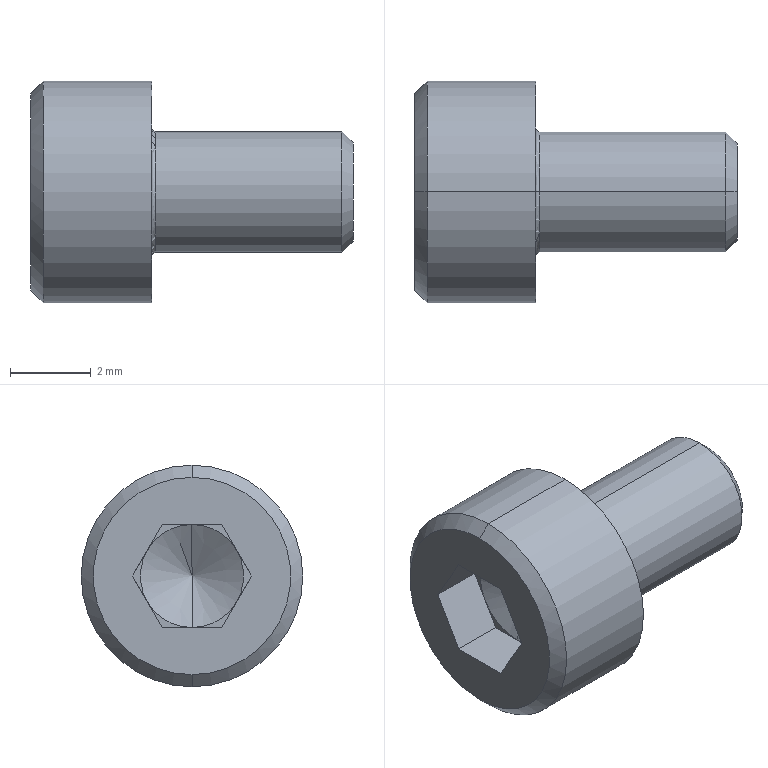Part | SolidWorks | features CirPattern 3, Cut 3, RevCut 2, Fillet 1, LPattern 1, Revolution 1 | 1 solid | 27 faces | box 8 x 5.5 x 5.5 mm | volume 96.895 mm3 | plane 15 | cone 6 | cylinder 4 | torus 2 | commonest cylinder face diameters 3 x2 5.5 x2
STEP:
#1=CARTESIAN_POINT('',(2.039,0.,0.));
#2=VERTEX_POINT('',#1);
#3=CARTESIAN_POINT('',(1.3,0.,1.28));
#4=VERTEX_POINT('',#3);
#5=CARTESIAN_POINT('',(1.3,0.,1.28));
#6=DIRECTION('',(-0.5,0.,0.866));
#7=VECTOR('',#6,1000.);
#8=LINE('',#5,#7);
#9=EDGE_CURVE('',#2,#4,#8,.T.);
#10=ORIENTED_EDGE('',*,*,#9,.F.);
#11=CARTESIAN_POINT('',(1.3,0.,-1.28));
#12=VERTEX_POINT('',#11);
#13=CARTESIAN_POINT('',(1.3,0.,-1.28));
#14=DIRECTION('',(-0.5,0.,-0.866));
#15=VECTOR('',#14,1000.);
#16=LINE('',#13,#15);
#17=EDGE_CURVE('',#2,#12,#16,.T.);
#18=ORIENTED_EDGE('',*,*,#17,.T.);
#19=CARTESIAN_POINT('',(1.3,-1.109,-0.64));
#20=VERTEX_POINT('',#19);
#21=CARTESIAN_POINT('',(1.3,0.,0.));
#22=DIRECTION('',(-1.,0.,0.));
#23=DIRECTION('',(0.,0.,1.));
#24=AXIS2_PLACEMENT_3D('',#21,#22,#23);
#25=CIRCLE('',#24,1.28);
#26=EDGE_CURVE('',#12,#20,#25,.T.);
#27=ORIENTED_EDGE('',*,*,#26,.T.);
#28=CARTESIAN_POINT('',(1.3,-1.109,0.64));
#29=VERTEX_POINT('',#28);
#30=CARTESIAN_POINT('',(1.3,0.,0.));
#31=DIRECTION('',(-1.,0.,0.));
#32=DIRECTION('',(0.,0.,1.));
#33=AXIS2_PLACEMENT_3D('',#30,#31,#32);
#34=CIRCLE('',#33,1.28);
#35=EDGE_CURVE('',#20,#29,#34,.T.);
#36=ORIENTED_EDGE('',*,*,#35,.T.);
#37=CARTESIAN_POINT('',(1.3,0.,0.));
#38=DIRECTION('',(-1.,0.,0.));
#39=DIRECTION('',(0.,0.,1.));
#40=AXIS2_PLACEMENT_3D('',#37,#38,#39);
#41=CIRCLE('',#40,1.28);
#42=EDGE_CURVE('',#29,#4,#41,.T.);
#43=ORIENTED_EDGE('',*,*,#42,.T.);
#44=EDGE_LOOP('',(#10,#18,#27,#36,#43));
#45=FACE_OUTER_BOUND('',#44,.T.);
#46=CARTESIAN_POINT('',(1.3,0.,0.));
#47=DIRECTION('',(-1.,0.,0.));
#48=DIRECTION('',(0.,0.,1.));
#49=AXIS2_PLACEMENT_3D('',#46,#47,#48);
#50=CONICAL_SURFACE('',#49,1.28,1.047);
#51=ADVANCED_FACE('',(#45),#50,.F.);
#52=CARTESIAN_POINT('',(3.1,0.,1.5));
#53=VERTEX_POINT('',#52);
#54=CARTESIAN_POINT('',(3.1,0.,-1.5));
#55=VERTEX_POINT('',#54);
#56=CARTESIAN_POINT('',(3.1,0.,0.));
#57=DIRECTION('',(1.,0.,0.));
#58=DIRECTION('',(0.,0.,-1.));
#59=AXIS2_PLACEMENT_3D('',#56,#57,#58);
#60=CIRCLE('',#59,1.5);
#61=EDGE_CURVE('',#53,#55,#60,.T.);
#62=ORIENTED_EDGE('',*,*,#61,.F.);
#63=CARTESIAN_POINT('',(3.,0.,1.6));
#64=VERTEX_POINT('',#63);
#65=CARTESIAN_POINT('',(3.1,0.,1.6));
#66=DIRECTION('',(0.,1.,0.));
#67=DIRECTION('',(0.,0.,1.));
#68=AXIS2_PLACEMENT_3D('',#65,#66,#67);
#69=CIRCLE('',#68,0.1);
#70=EDGE_CURVE('',#53,#64,#69,.T.);
#71=ORIENTED_EDGE('',*,*,#70,.T.);
#72=CARTESIAN_POINT('',(3.,0.,-1.6));
#73=VERTEX_POINT('',#72);
#74=CARTESIAN_POINT('',(3.,0.,0.));
#75=DIRECTION('',(-1.,0.,0.));
#76=DIRECTION('',(0.,0.,-1.));
#77=AXIS2_PLACEMENT_3D('',#74,#75,#76);
#78=CIRCLE('',#77,1.6);
#79=EDGE_CURVE('',#73,#64,#78,.T.);
#80=ORIENTED_EDGE('',*,*,#79,.F.);
#81=CARTESIAN_POINT('',(3.1,0.,-1.6));
#82=DIRECTION('',(0.,-1.,0.));
#83=DIRECTION('',(0.,0.,-1.));
#84=AXIS2_PLACEMENT_3D('',#81,#82,#83);
#85=CIRCLE('',#84,0.1);
#86=EDGE_CURVE('',#55,#73,#85,.T.);
#87=ORIENTED_EDGE('',*,*,#86,.F.);
#88=EDGE_LOOP('',(#62,#71,#80,#87));
#89=FACE_OUTER_BOUND('',#88,.T.);
#90=CARTESIAN_POINT('',(3.1,0.,0.));
#91=DIRECTION('',(1.,0.,0.));
#92=DIRECTION('',(0.,0.,-1.));
#93=AXIS2_PLACEMENT_3D('',#90,#91,#92);
#94=TOROIDAL_SURFACE('',#93,1.6,0.1);
#95=ADVANCED_FACE('',(#89),#94,.F.);
#96=CARTESIAN_POINT('',(0.,0.,2.45));
#97=VERTEX_POINT('',#96);
#98=CARTESIAN_POINT('',(0.,0.,-2.45));
#99=VERTEX_POINT('',#98);
#100=CARTESIAN_POINT('',(0.,0.,0.));
#101=DIRECTION('',(-1.,0.,0.));
#102=DIRECTION('',(0.,0.,1.));
#103=AXIS2_PLACEMENT_3D('',#100,#101,#102);
#104=CIRCLE('',#103,2.45);
#105=EDGE_CURVE('',#97,#99,#104,.T.);
#106=ORIENTED_EDGE('',*,*,#105,.F.);
#107=CARTESIAN_POINT('',(0.3,0.,2.75));
#108=VERTEX_POINT('',#107);
#109=CARTESIAN_POINT('',(0.,0.,2.45));
#110=DIRECTION('',(0.7071,0.,0.7071));
#111=VECTOR('',#110,1000.);
#112=LINE('',#109,#111);
#113=EDGE_CURVE('',#97,#108,#112,.T.);
#114=ORIENTED_EDGE('',*,*,#113,.T.);
#115=CARTESIAN_POINT('',(0.3,0.,-2.75));
#116=VERTEX_POINT('',#115);
#117=CARTESIAN_POINT('',(0.3,0.,0.));
#118=DIRECTION('',(-1.,0.,0.));
#119=DIRECTION('',(0.,0.,1.));
#120=AXIS2_PLACEMENT_3D('',#117,#118,#119);
#121=CIRCLE('',#120,2.75);
#122=EDGE_CURVE('',#108,#116,#121,.T.);
#123=ORIENTED_EDGE('',*,*,#122,.T.);
#124=CARTESIAN_POINT('',(0.,0.,-2.45));
#125=DIRECTION('',(0.7071,0.,-0.7071));
#126=VECTOR('',#125,1000.);
#127=LINE('',#124,#126);
#128=EDGE_CURVE('',#99,#116,#127,.T.);
#129=ORIENTED_EDGE('',*,*,#128,.F.);
#130=EDGE_LOOP('',(#106,#114,#123,#129));
#131=FACE_OUTER_BOUND('',#130,.T.);
#132=CARTESIAN_POINT('',(0.,0.,0.));
#133=DIRECTION('',(1.,0.,0.));
#134=DIRECTION('',(0.,0.,-1.));
#135=AXIS2_PLACEMENT_3D('',#132,#133,#134);
#136=CONICAL_SURFACE('',#135,2.45,0.7854);
#137=ADVANCED_FACE('',(#131),#136,.T.);
#138=CARTESIAN_POINT('',(3.,0.,2.75));
#139=VERTEX_POINT('',#138);
#140=CARTESIAN_POINT('',(3.,0.,-2.75));
#141=VERTEX_POINT('',#140);
#142=CARTESIAN_POINT('',(3.,0.,0.));
#143=DIRECTION('',(-1.,0.,0.));
#144=DIRECTION('',(0.,0.,1.));
#145=AXIS2_PLACEMENT_3D('',#142,#143,#144);
#146=CIRCLE('',#145,2.75);
#147=EDGE_CURVE('',#139,#141,#146,.T.);
#148=ORIENTED_EDGE('',*,*,#147,.T.);
#149=CARTESIAN_POINT('',(-31.75,0.,-2.75));
#150=DIRECTION('',(-1.,0.,0.));
#151=VECTOR('',#150,1000.);
#152=LINE('',#149,#151);
#153=EDGE_CURVE('',#141,#116,#152,.T.);
#154=ORIENTED_EDGE('',*,*,#153,.T.);
#155=ORIENTED_EDGE('',*,*,#122,.F.);
#156=CARTESIAN_POINT('',(-31.75,0.,2.75));
#157=DIRECTION('',(-1.,0.,0.));
#158=VECTOR('',#157,1000.);
#159=LINE('',#156,#158);
#160=EDGE_CURVE('',#139,#108,#159,.T.);
#161=ORIENTED_EDGE('',*,*,#160,.F.);
#162=EDGE_LOOP('',(#148,#154,#155,#161));
#163=FACE_OUTER_BOUND('',#162,.T.);
#164=CARTESIAN_POINT('',(-31.75,0.,0.));
#165=DIRECTION('',(-1.,0.,0.));
#166=DIRECTION('',(0.,0.,1.));
#167=AXIS2_PLACEMENT_3D('',#164,#165,#166);
#168=CYLINDRICAL_SURFACE('',#167,2.75);
#169=ADVANCED_FACE('',(#163),#168,.T.);
#170=CARTESIAN_POINT('',(7.72,0.,1.5));
#171=VERTEX_POINT('',#170);
#172=CARTESIAN_POINT('',(7.72,0.,-1.5));
#173=VERTEX_POINT('',#172);
#174=CARTESIAN_POINT('',(7.72,0.,0.));
#175=DIRECTION('',(-1.,0.,0.));
#176=DIRECTION('',(0.,0.,1.));
#177=AXIS2_PLACEMENT_3D('',#174,#175,#176);
#178=CIRCLE('',#177,1.5);
#179=EDGE_CURVE('',#171,#173,#178,.T.);
#180=ORIENTED_EDGE('',*,*,#179,.T.);
#181=CARTESIAN_POINT('',(-31.75,0.,-1.5));
#182=DIRECTION('',(-1.,0.,0.));
#183=VECTOR('',#182,1000.);
#184=LINE('',#181,#183);
#185=EDGE_CURVE('',#173,#55,#184,.T.);
#186=ORIENTED_EDGE('',*,*,#185,.T.);
#187=CARTESIAN_POINT('',(3.1,0.,0.));
#188=DIRECTION('',(1.,0.,0.));
#189=DIRECTION('',(0.,0.,-1.));
#190=AXIS2_PLACEMENT_3D('',#187,#188,#189);
#191=CIRCLE('',#190,1.5);
#192=EDGE_CURVE('',#55,#53,#191,.T.);
#193=ORIENTED_EDGE('',*,*,#192,.T.);
#194=CARTESIAN_POINT('',(-31.75,0.,1.5));
#195=DIRECTION('',(-1.,0.,0.));
#196=VECTOR('',#195,1000.);
#197=LINE('',#194,#196);
#198=EDGE_CURVE('',#171,#53,#197,.T.);
#199=ORIENTED_EDGE('',*,*,#198,.F.);
#200=EDGE_LOOP('',(#180,#186,#193,#199));
#201=FACE_OUTER_BOUND('',#200,.T.);
#202=CARTESIAN_POINT('',(-31.75,0.,0.));
#203=DIRECTION('',(-1.,0.,0.));
#204=DIRECTION('',(0.,0.,1.));
#205=AXIS2_PLACEMENT_3D('',#202,#203,#204);
#206=CYLINDRICAL_SURFACE('',#205,1.5);
#207=ADVANCED_FACE('',(#201),#206,.T.);
#208=CARTESIAN_POINT('',(8.,0.,1.22));
#209=VERTEX_POINT('',#208);
#210=CARTESIAN_POINT('',(8.,0.,-1.22));
#211=VERTEX_POINT('',#210);
#212=CARTESIAN_POINT('',(8.,0.,0.));
#213=DIRECTION('',(-1.,0.,0.));
#214=DIRECTION('',(0.,0.,1.));
#215=AXIS2_PLACEMENT_3D('',#212,#213,#214);
#216=CIRCLE('',#215,1.22);
#217=EDGE_CURVE('',#209,#211,#216,.T.);
#218=ORIENTED_EDGE('',*,*,#217,.T.);
#219=CARTESIAN_POINT('',(8.,0.,-1.22));
#220=DIRECTION('',(-0.7071,0.,-0.7071));
#221=VECTOR('',#220,1000.);
#222=LINE('',#219,#221);
#223=EDGE_CURVE('',#211,#173,#222,.T.);
#224=ORIENTED_EDGE('',*,*,#223,.T.);
#225=ORIENTED_EDGE('',*,*,#179,.F.);
#226=CARTESIAN_POINT('',(8.,0.,1.22));
#227=DIRECTION('',(-0.7071,0.,0.7071));
#228=VECTOR('',#227,1000.);
#229=LINE('',#226,#228);
#230=EDGE_CURVE('',#209,#171,#229,.T.);
#231=ORIENTED_EDGE('',*,*,#230,.F.);
#232=EDGE_LOOP('',(#218,#224,#225,#231));
#233=FACE_OUTER_BOUND('',#232,.T.);
#234=CARTESIAN_POINT('',(8.,0.,0.));
#235=DIRECTION('',(-1.,0.,0.));
#236=DIRECTION('',(0.,0.,1.));
#237=AXIS2_PLACEMENT_3D('',#234,#235,#236);
#238=CONICAL_SURFACE('',#237,1.22,0.7854);
#239=ADVANCED_FACE('',(#233),#238,.T.);
#240=CARTESIAN_POINT('',(0.,1.478,0.));
#241=VERTEX_POINT('',#240);
#242=CARTESIAN_POINT('',(0.,0.739,1.28));
#243=VERTEX_POINT('',#242);
#244=CARTESIAN_POINT('',(0.,1.478,0.));
#245=DIRECTION('',(0.,-0.5,0.866));
#246=VECTOR('',#245,1000.);
#247=LINE('',#244,#246);
#248=EDGE_CURVE('',#241,#243,#247,.T.);
#249=ORIENTED_EDGE('',*,*,#248,.T.);
#250=CARTESIAN_POINT('',(0.,-0.739,1.28));
#251=VERTEX_POINT('',#250);
#252=CARTESIAN_POINT('',(0.,-0.739,1.28));
#253=DIRECTION('',(0.,1.,0.));
#254=VECTOR('',#253,1000.);
#255=LINE('',#252,#254);
#256=EDGE_CURVE('',#251,#243,#255,.T.);
#257=ORIENTED_EDGE('',*,*,#256,.F.);
#258=CARTESIAN_POINT('',(0.,-1.478,0.));
#259=VERTEX_POINT('',#258);
#260=CARTESIAN_POINT('',(0.,-0.739,1.28));
#261=DIRECTION('',(0.,-0.5,-0.866));
#262=VECTOR('',#261,1000.);
#263=LINE('',#260,#262);
#264=EDGE_CURVE('',#251,#259,#263,.T.);
#265=ORIENTED_EDGE('',*,*,#264,.T.);
#266=CARTESIAN_POINT('',(0.,-0.739,-1.28));
#267=VERTEX_POINT('',#266);
#268=CARTESIAN_POINT('',(0.,-1.478,0.));
#269=DIRECTION('',(0.,0.5,-0.866));
#270=VECTOR('',#269,1000.);
#271=LINE('',#268,#270);
#272=EDGE_CURVE('',#259,#267,#271,.T.);
#273=ORIENTED_EDGE('',*,*,#272,.T.);
#274=CARTESIAN_POINT('',(0.,0.739,-1.28));
#275=VERTEX_POINT('',#274);
#276=CARTESIAN_POINT('',(0.,0.739,-1.28));
#277=DIRECTION('',(0.,-1.,0.));
#278=VECTOR('',#277,1000.);
#279=LINE('',#276,#278);
#280=EDGE_CURVE('',#275,#267,#279,.T.);
#281=ORIENTED_EDGE('',*,*,#280,.F.);
#282=CARTESIAN_POINT('',(0.,1.478,0.));
#283=DIRECTION('',(0.,-0.5,-0.866));
#284=VECTOR('',#283,1000.);
#285=LINE('',#282,#284);
#286=EDGE_CURVE('',#241,#275,#285,.T.);
#287=ORIENTED_EDGE('',*,*,#286,.F.);
#288=EDGE_LOOP('',(#249,#257,#265,#273,#281,#287));
#289=FACE_BOUND('',#288,.T.);
#290=CARTESIAN_POINT('',(0.,0.,0.));
#291=DIRECTION('',(-1.,0.,0.));
#292=DIRECTION('',(0.,0.,1.));
#293=AXIS2_PLACEMENT_3D('',#290,#291,#292);
#294=CIRCLE('',#293,2.45);
#295=EDGE_CURVE('',#99,#97,#294,.T.);
#296=ORIENTED_EDGE('',*,*,#295,.T.);
#297=ORIENTED_EDGE('',*,*,#105,.T.);
#298=EDGE_LOOP('',(#296,#297));
#299=FACE_OUTER_BOUND('',#298,.T.);
#300=CARTESIAN_POINT('',(0.,0.,0.));
#301=DIRECTION('',(-1.,0.,0.));
#302=DIRECTION('',(0.,0.,1.));
#303=AXIS2_PLACEMENT_3D('',#300,#301,#302);
#304=PLANE('',#303);
#305=ADVANCED_FACE('',(#289,#299),#304,.T.);
#306=ORIENTED_EDGE('',*,*,#217,.F.);
#307=CARTESIAN_POINT('',(8.,0.,0.));
#308=DIRECTION('',(-1.,0.,0.));
#309=DIRECTION('',(0.,0.,1.));
#310=AXIS2_PLACEMENT_3D('',#307,#308,#309);
#311=CIRCLE('',#310,1.22);
#312=EDGE_CURVE('',#211,#209,#311,.T.);
#313=ORIENTED_EDGE('',*,*,#312,.F.);
#314=EDGE_LOOP('',(#306,#313));
#315=FACE_OUTER_BOUND('',#314,.T.);
#316=CARTESIAN_POINT('',(8.,1.22,0.));
#317=DIRECTION('',(1.,0.,0.));
#318=DIRECTION('',(0.,0.,-1.));
#319=AXIS2_PLACEMENT_3D('',#316,#317,#318);
#320=PLANE('',#319);
#321=ADVANCED_FACE('',(#315),#320,.T.);
#322=ORIENTED_EDGE('',*,*,#223,.F.);
#323=ORIENTED_EDGE('',*,*,#312,.T.);
#324=ORIENTED_EDGE('',*,*,#230,.T.);
#325=CARTESIAN_POINT('',(7.72,0.,0.));
#326=DIRECTION('',(-1.,0.,0.));
#327=DIRECTION('',(0.,0.,1.));
#328=AXIS2_PLACEMENT_3D('',#325,#326,#327);
#329=CIRCLE('',#328,1.5);
#330=EDGE_CURVE('',#173,#171,#329,.T.);
#331=ORIENTED_EDGE('',*,*,#330,.F.);
#332=EDGE_LOOP('',(#322,#323,#324,#331));
#333=FACE_OUTER_BOUND('',#332,.T.);
#334=CARTESIAN_POINT('',(8.,0.,0.));
#335=DIRECTION('',(-1.,0.,0.));
#336=DIRECTION('',(0.,0.,1.));
#337=AXIS2_PLACEMENT_3D('',#334,#335,#336);
#338=CONICAL_SURFACE('',#337,1.22,0.7854);
#339=ADVANCED_FACE('',(#333),#338,.T.);
#340=ORIENTED_EDGE('',*,*,#185,.F.);
#341=ORIENTED_EDGE('',*,*,#330,.T.);
#342=ORIENTED_EDGE('',*,*,#198,.T.);
#343=ORIENTED_EDGE('',*,*,#61,.T.);
#344=EDGE_LOOP('',(#340,#341,#342,#343));
#345=FACE_OUTER_BOUND('',#344,.T.);
#346=CARTESIAN_POINT('',(-31.75,0.,0.));
#347=DIRECTION('',(-1.,0.,0.));
#348=DIRECTION('',(0.,0.,1.));
#349=AXIS2_PLACEMENT_3D('',#346,#347,#348);
#350=CYLINDRICAL_SURFACE('',#349,1.5);
#351=ADVANCED_FACE('',(#345),#350,.T.);
#352=ORIENTED_EDGE('',*,*,#79,.T.);
#353=CARTESIAN_POINT('',(3.,0.,0.));
#354=DIRECTION('',(-1.,0.,0.));
#355=DIRECTION('',(0.,0.,-1.));
#356=AXIS2_PLACEMENT_3D('',#353,#354,#355);
#357=CIRCLE('',#356,1.6);
#358=EDGE_CURVE('',#64,#73,#357,.T.);
#359=ORIENTED_EDGE('',*,*,#358,.T.);
#360=EDGE_LOOP('',(#352,#359));
#361=FACE_BOUND('',#360,.T.);
#362=ORIENTED_EDGE('',*,*,#147,.F.);
#363=CARTESIAN_POINT('',(3.,0.,0.));
#364=DIRECTION('',(-1.,0.,0.));
#365=DIRECTION('',(0.,0.,1.));
#366=AXIS2_PLACEMENT_3D('',#363,#364,#365);
#367=CIRCLE('',#366,2.75);
#368=EDGE_CURVE('',#141,#139,#367,.T.);
#369=ORIENTED_EDGE('',*,*,#368,.F.);
#370=EDGE_LOOP('',(#362,#369));
#371=FACE_OUTER_BOUND('',#370,.T.);
#372=CARTESIAN_POINT('',(3.,2.75,0.));
#373=DIRECTION('',(1.,0.,0.));
#374=DIRECTION('',(0.,0.,-1.));
#375=AXIS2_PLACEMENT_3D('',#372,#373,#374);
#376=PLANE('',#375);
#377=ADVANCED_FACE('',(#361,#371),#376,.T.);
#378=ORIENTED_EDGE('',*,*,#153,.F.);
#379=ORIENTED_EDGE('',*,*,#368,.T.);
#380=ORIENTED_EDGE('',*,*,#160,.T.);
#381=CARTESIAN_POINT('',(0.3,0.,0.));
#382=DIRECTION('',(-1.,0.,0.));
#383=DIRECTION('',(0.,0.,1.));
#384=AXIS2_PLACEMENT_3D('',#381,#382,#383);
#385=CIRCLE('',#384,2.75);
#386=EDGE_CURVE('',#116,#108,#385,.T.);
#387=ORIENTED_EDGE('',*,*,#386,.F.);
#388=EDGE_LOOP('',(#378,#379,#380,#387));
#389=FACE_OUTER_BOUND('',#388,.T.);
#390=CARTESIAN_POINT('',(-31.75,0.,0.));
#391=DIRECTION('',(-1.,0.,0.));
#392=DIRECTION('',(0.,0.,1.));
#393=AXIS2_PLACEMENT_3D('',#390,#391,#392);
#394=CYLINDRICAL_SURFACE('',#393,2.75);
#395=ADVANCED_FACE('',(#389),#394,.T.);
#396=ORIENTED_EDGE('',*,*,#113,.F.);
#397=ORIENTED_EDGE('',*,*,#295,.F.);
#398=ORIENTED_EDGE('',*,*,#128,.T.);
#399=ORIENTED_EDGE('',*,*,#386,.T.);
#400=EDGE_LOOP('',(#396,#397,#398,#399));
#401=FACE_OUTER_BOUND('',#400,.T.);
#402=CARTESIAN_POINT('',(0.,0.,0.));
#403=DIRECTION('',(1.,0.,0.));
#404=DIRECTION('',(0.,0.,-1.));
#405=AXIS2_PLACEMENT_3D('',#402,#403,#404);
#406=CONICAL_SURFACE('',#405,2.45,0.7854);
#407=ADVANCED_FACE('',(#401),#406,.T.);
#408=ORIENTED_EDGE('',*,*,#70,.F.);
#409=ORIENTED_EDGE('',*,*,#192,.F.);
#410=ORIENTED_EDGE('',*,*,#86,.T.);
#411=ORIENTED_EDGE('',*,*,#358,.F.);
#412=EDGE_LOOP('',(#408,#409,#410,#411));
#413=FACE_OUTER_BOUND('',#412,.T.);
#414=CARTESIAN_POINT('',(3.1,0.,0.));
#415=DIRECTION('',(1.,0.,0.));
#416=DIRECTION('',(0.,0.,-1.));
#417=AXIS2_PLACEMENT_3D('',#414,#415,#416);
#418=TOROIDAL_SURFACE('',#417,1.6,0.1);
#419=ADVANCED_FACE('',(#413),#418,.F.);
#420=ORIENTED_EDGE('',*,*,#248,.F.);
#421=CARTESIAN_POINT('',(1.3,1.478,0.));
#422=VERTEX_POINT('',#421);
#423=CARTESIAN_POINT('',(1.3,1.478,0.));
#424=DIRECTION('',(-1.,0.,0.));
#425=VECTOR('',#424,1000.);
#426=LINE('',#423,#425);
#427=EDGE_CURVE('',#422,#241,#426,.T.);
#428=ORIENTED_EDGE('',*,*,#427,.F.);
#429=CARTESIAN_POINT('',(1.3,1.109,0.64));
#430=VERTEX_POINT('',#429);
#431=CARTESIAN_POINT('',(1.3,1.478,0.));
#432=DIRECTION('',(0.,-0.5,0.866));
#433=VECTOR('',#432,1000.);
#434=LINE('',#431,#433);
#435=EDGE_CURVE('',#422,#430,#434,.T.);
#436=ORIENTED_EDGE('',*,*,#435,.T.);
#437=CARTESIAN_POINT('',(1.3,0.739,1.28));
#438=VERTEX_POINT('',#437);
#439=CARTESIAN_POINT('',(1.3,1.478,0.));
#440=DIRECTION('',(0.,-0.5,0.866));
#441=VECTOR('',#440,1000.);
#442=LINE('',#439,#441);
#443=EDGE_CURVE('',#430,#438,#442,.T.);
#444=ORIENTED_EDGE('',*,*,#443,.T.);
#445=CARTESIAN_POINT('',(1.3,0.739,1.28));
#446=DIRECTION('',(-1.,0.,0.));
#447=VECTOR('',#446,1000.);
#448=LINE('',#445,#447);
#449=EDGE_CURVE('',#438,#243,#448,.T.);
#450=ORIENTED_EDGE('',*,*,#449,.T.);
#451=EDGE_LOOP('',(#420,#428,#436,#444,#450));
#452=FACE_OUTER_BOUND('',#451,.T.);
#453=CARTESIAN_POINT('',(1.3,1.478,0.));
#454=DIRECTION('',(0.,-0.866,-0.5));
#455=DIRECTION('',(0.,0.5,-0.866));
#456=AXIS2_PLACEMENT_3D('',#453,#454,#455);
#457=PLANE('',#456);
#458=ADVANCED_FACE('',(#452),#457,.T.);
#459=ORIENTED_EDGE('',*,*,#256,.T.);
#460=ORIENTED_EDGE('',*,*,#449,.F.);
#461=CARTESIAN_POINT('',(1.3,-0.739,1.28));
#462=DIRECTION('',(0.,1.,0.));
#463=VECTOR('',#462,1000.);
#464=LINE('',#461,#463);
#465=EDGE_CURVE('',#4,#438,#464,.T.);
#466=ORIENTED_EDGE('',*,*,#465,.F.);
#467=CARTESIAN_POINT('',(1.3,-0.739,1.28));
#468=VERTEX_POINT('',#467);
#469=CARTESIAN_POINT('',(1.3,-0.739,1.28));
#470=DIRECTION('',(0.,1.,0.));
#471=VECTOR('',#470,1000.);
#472=LINE('',#469,#471);
#473=EDGE_CURVE('',#468,#4,#472,.T.);
#474=ORIENTED_EDGE('',*,*,#473,.F.);
#475=CARTESIAN_POINT('',(1.3,-0.739,1.28));
#476=DIRECTION('',(-1.,0.,0.));
#477=VECTOR('',#476,1000.);
#478=LINE('',#475,#477);
#479=EDGE_CURVE('',#468,#251,#478,.T.);
#480=ORIENTED_EDGE('',*,*,#479,.T.);
#481=EDGE_LOOP('',(#459,#460,#466,#474,#480));
#482=FACE_OUTER_BOUND('',#481,.T.);
#483=CARTESIAN_POINT('',(1.3,-0.739,1.28));
#484=DIRECTION('',(0.,0.,1.));
#485=DIRECTION('',(0.,-1.,0.));
#486=AXIS2_PLACEMENT_3D('',#483,#484,#485);
#487=PLANE('',#486);
#488=ADVANCED_FACE('',(#482),#487,.F.);
#489=ORIENTED_EDGE('',*,*,#264,.F.);
#490=ORIENTED_EDGE('',*,*,#479,.F.);
#491=CARTESIAN_POINT('',(1.3,-0.739,1.28));
#492=DIRECTION('',(0.,-0.5,-0.866));
#493=VECTOR('',#492,1000.);
#494=LINE('',#491,#493);
#495=EDGE_CURVE('',#468,#29,#494,.T.);
#496=ORIENTED_EDGE('',*,*,#495,.T.);
#497=CARTESIAN_POINT('',(1.3,-1.478,0.));
#498=VERTEX_POINT('',#497);
#499=CARTESIAN_POINT('',(1.3,-0.739,1.28));
#500=DIRECTION('',(0.,-0.5,-0.866));
#501=VECTOR('',#500,1000.);
#502=LINE('',#499,#501);
#503=EDGE_CURVE('',#29,#498,#502,.T.);
#504=ORIENTED_EDGE('',*,*,#503,.T.);
#505=CARTESIAN_POINT('',(1.3,-1.478,0.));
#506=DIRECTION('',(-1.,0.,0.));
#507=VECTOR('',#506,1000.);
#508=LINE('',#505,#507);
#509=EDGE_CURVE('',#498,#259,#508,.T.);
#510=ORIENTED_EDGE('',*,*,#509,.T.);
#511=EDGE_LOOP('',(#489,#490,#496,#504,#510));
#512=FACE_OUTER_BOUND('',#511,.T.);
#513=CARTESIAN_POINT('',(1.3,-0.739,1.28));
#514=DIRECTION('',(0.,0.866,-0.5));
#515=DIRECTION('',(0.,0.5,0.866));
#516=AXIS2_PLACEMENT_3D('',#513,#514,#515);
#517=PLANE('',#516);
#518=ADVANCED_FACE('',(#512),#517,.T.);
#519=ORIENTED_EDGE('',*,*,#272,.F.);
#520=ORIENTED_EDGE('',*,*,#509,.F.);
#521=CARTESIAN_POINT('',(1.3,-1.478,0.));
#522=DIRECTION('',(0.,0.5,-0.866));
#523=VECTOR('',#522,1000.);
#524=LINE('',#521,#523);
#525=EDGE_CURVE('',#498,#20,#524,.T.);
#526=ORIENTED_EDGE('',*,*,#525,.T.);
#527=CARTESIAN_POINT('',(1.3,-0.739,-1.28));
#528=VERTEX_POINT('',#527);
#529=CARTESIAN_POINT('',(1.3,-1.478,0.));
#530=DIRECTION('',(0.,0.5,-0.866));
#531=VECTOR('',#530,1000.);
#532=LINE('',#529,#531);
#533=EDGE_CURVE('',#20,#528,#532,.T.);
#534=ORIENTED_EDGE('',*,*,#533,.T.);
#535=CARTESIAN_POINT('',(1.3,-0.739,-1.28));
#536=DIRECTION('',(-1.,0.,0.));
#537=VECTOR('',#536,1000.);
#538=LINE('',#535,#537);
#539=EDGE_CURVE('',#528,#267,#538,.T.);
#540=ORIENTED_EDGE('',*,*,#539,.T.);
#541=EDGE_LOOP('',(#519,#520,#526,#534,#540));
#542=FACE_OUTER_BOUND('',#541,.T.);
#543=CARTESIAN_POINT('',(1.3,-1.478,0.));
#544=DIRECTION('',(0.,0.866,0.5));
#545=DIRECTION('',(0.,-0.5,0.866));
#546=AXIS2_PLACEMENT_3D('',#543,#544,#545);
#547=PLANE('',#546);
#548=ADVANCED_FACE('',(#542),#547,.T.);
#549=ORIENTED_EDGE('',*,*,#280,.T.);
#550=ORIENTED_EDGE('',*,*,#539,.F.);
#551=CARTESIAN_POINT('',(1.3,0.739,-1.28));
#552=DIRECTION('',(0.,-1.,0.));
#553=VECTOR('',#552,1000.);
#554=LINE('',#551,#553);
#555=EDGE_CURVE('',#12,#528,#554,.T.);
#556=ORIENTED_EDGE('',*,*,#555,.F.);
#557=CARTESIAN_POINT('',(1.3,0.739,-1.28));
#558=VERTEX_POINT('',#557);
#559=CARTESIAN_POINT('',(1.3,0.739,-1.28));
#560=DIRECTION('',(0.,-1.,0.));
#561=VECTOR('',#560,1000.);
#562=LINE('',#559,#561);
#563=EDGE_CURVE('',#558,#12,#562,.T.);
#564=ORIENTED_EDGE('',*,*,#563,.F.);
#565=CARTESIAN_POINT('',(1.3,0.739,-1.28));
#566=DIRECTION('',(-1.,0.,0.));
#567=VECTOR('',#566,1000.);
#568=LINE('',#565,#567);
#569=EDGE_CURVE('',#558,#275,#568,.T.);
#570=ORIENTED_EDGE('',*,*,#569,.T.);
#571=EDGE_LOOP('',(#549,#550,#556,#564,#570));
#572=FACE_OUTER_BOUND('',#571,.T.);
#573=CARTESIAN_POINT('',(1.3,0.739,-1.28));
#574=DIRECTION('',(0.,0.,-1.));
#575=DIRECTION('',(0.,1.,0.));
#576=AXIS2_PLACEMENT_3D('',#573,#574,#575);
#577=PLANE('',#576);
#578=ADVANCED_FACE('',(#572),#577,.F.);
#579=ORIENTED_EDGE('',*,*,#286,.T.);
#580=ORIENTED_EDGE('',*,*,#569,.F.);
#581=CARTESIAN_POINT('',(1.3,1.109,-0.64));
#582=VERTEX_POINT('',#581);
#583=CARTESIAN_POINT('',(1.3,1.478,0.));
#584=DIRECTION('',(0.,-0.5,-0.866));
#585=VECTOR('',#584,1000.);
#586=LINE('',#583,#585);
#587=EDGE_CURVE('',#582,#558,#586,.T.);
#588=ORIENTED_EDGE('',*,*,#587,.F.);
#589=CARTESIAN_POINT('',(1.3,1.478,0.));
#590=DIRECTION('',(0.,-0.5,-0.866));
#591=VECTOR('',#590,1000.);
#592=LINE('',#589,#591);
#593=EDGE_CURVE('',#422,#582,#592,.T.);
#594=ORIENTED_EDGE('',*,*,#593,.F.);
#595=ORIENTED_EDGE('',*,*,#427,.T.);
#596=EDGE_LOOP('',(#579,#580,#588,#594,#595));
#597=FACE_OUTER_BOUND('',#596,.T.);
#598=CARTESIAN_POINT('',(1.3,1.478,0.));
#599=DIRECTION('',(0.,0.866,-0.5));
#600=DIRECTION('',(0.,0.5,0.866));
#601=AXIS2_PLACEMENT_3D('',#598,#599,#600);
#602=PLANE('',#601);
#603=ADVANCED_FACE('',(#597),#602,.F.);
#604=ORIENTED_EDGE('',*,*,#555,.T.);
#605=ORIENTED_EDGE('',*,*,#533,.F.);
#606=ORIENTED_EDGE('',*,*,#26,.F.);
#607=EDGE_LOOP('',(#604,#605,#606));
#608=FACE_OUTER_BOUND('',#607,.T.);
#609=CARTESIAN_POINT('',(1.3,1.478,0.));
#610=DIRECTION('',(1.,0.,0.));
#611=DIRECTION('',(0.,0.,-1.));
#612=AXIS2_PLACEMENT_3D('',#609,#610,#611);
#613=PLANE('',#612);
#614=ADVANCED_FACE('',(#608),#613,.F.);
#615=ORIENTED_EDGE('',*,*,#525,.F.);
#616=ORIENTED_EDGE('',*,*,#503,.F.);
#617=ORIENTED_EDGE('',*,*,#35,.F.);
#618=EDGE_LOOP('',(#615,#616,#617));
#619=FACE_OUTER_BOUND('',#618,.T.);
#620=CARTESIAN_POINT('',(1.3,1.478,0.));
#621=DIRECTION('',(1.,0.,0.));
#622=DIRECTION('',(0.,0.,-1.));
#623=AXIS2_PLACEMENT_3D('',#620,#621,#622);
#624=PLANE('',#623);
#625=ADVANCED_FACE('',(#619),#624,.F.);
#626=ORIENTED_EDGE('',*,*,#495,.F.);
#627=ORIENTED_EDGE('',*,*,#473,.T.);
#628=ORIENTED_EDGE('',*,*,#42,.F.);
#629=EDGE_LOOP('',(#626,#627,#628));
#630=FACE_OUTER_BOUND('',#629,.T.);
#631=CARTESIAN_POINT('',(1.3,1.478,0.));
#632=DIRECTION('',(1.,0.,0.));
#633=DIRECTION('',(0.,0.,-1.));
#634=AXIS2_PLACEMENT_3D('',#631,#632,#633);
#635=PLANE('',#634);
#636=ADVANCED_FACE('',(#630),#635,.F.);
#637=ORIENTED_EDGE('',*,*,#465,.T.);
#638=ORIENTED_EDGE('',*,*,#443,.F.);
#639=CARTESIAN_POINT('',(1.3,0.,0.));
#640=DIRECTION('',(-1.,0.,0.));
#641=DIRECTION('',(0.,0.,1.));
#642=AXIS2_PLACEMENT_3D('',#639,#640,#641);
#643=CIRCLE('',#642,1.28);
#644=EDGE_CURVE('',#4,#430,#643,.T.);
#645=ORIENTED_EDGE('',*,*,#644,.F.);
#646=EDGE_LOOP('',(#637,#638,#645));
#647=FACE_OUTER_BOUND('',#646,.T.);
#648=CARTESIAN_POINT('',(1.3,1.478,0.));
#649=DIRECTION('',(1.,0.,0.));
#650=DIRECTION('',(0.,0.,-1.));
#651=AXIS2_PLACEMENT_3D('',#648,#649,#650);
#652=PLANE('',#651);
#653=ADVANCED_FACE('',(#647),#652,.F.);
#654=ORIENTED_EDGE('',*,*,#435,.F.);
#655=ORIENTED_EDGE('',*,*,#593,.T.);
#656=CARTESIAN_POINT('',(1.3,0.,0.));
#657=DIRECTION('',(-1.,0.,0.));
#658=DIRECTION('',(0.,0.,1.));
#659=AXIS2_PLACEMENT_3D('',#656,#657,#658);
#660=CIRCLE('',#659,1.28);
#661=EDGE_CURVE('',#430,#582,#660,.T.);
#662=ORIENTED_EDGE('',*,*,#661,.F.);
#663=EDGE_LOOP('',(#654,#655,#662));
#664=FACE_OUTER_BOUND('',#663,.T.);
#665=CARTESIAN_POINT('',(1.3,1.478,0.));
#666=DIRECTION('',(1.,0.,0.));
#667=DIRECTION('',(0.,0.,-1.));
#668=AXIS2_PLACEMENT_3D('',#665,#666,#667);
#669=PLANE('',#668);
#670=ADVANCED_FACE('',(#664),#669,.F.);
#671=ORIENTED_EDGE('',*,*,#587,.T.);
#672=ORIENTED_EDGE('',*,*,#563,.T.);
#673=CARTESIAN_POINT('',(1.3,0.,0.));
#674=DIRECTION('',(-1.,0.,0.));
#675=DIRECTION('',(0.,0.,1.));
#676=AXIS2_PLACEMENT_3D('',#673,#674,#675);
#677=CIRCLE('',#676,1.28);
#678=EDGE_CURVE('',#582,#12,#677,.T.);
#679=ORIENTED_EDGE('',*,*,#678,.F.);
#680=EDGE_LOOP('',(#671,#672,#679));
#681=FACE_OUTER_BOUND('',#680,.T.);
#682=CARTESIAN_POINT('',(1.3,1.478,0.));
#683=DIRECTION('',(1.,0.,0.));
#684=DIRECTION('',(0.,0.,-1.));
#685=AXIS2_PLACEMENT_3D('',#682,#683,#684);
#686=PLANE('',#685);
#687=ADVANCED_FACE('',(#681),#686,.F.);
#688=ORIENTED_EDGE('',*,*,#17,.F.);
#689=ORIENTED_EDGE('',*,*,#9,.T.);
#690=ORIENTED_EDGE('',*,*,#644,.T.);
#691=ORIENTED_EDGE('',*,*,#661,.T.);
#692=ORIENTED_EDGE('',*,*,#678,.T.);
#693=EDGE_LOOP('',(#688,#689,#690,#691,#692));
#694=FACE_OUTER_BOUND('',#693,.T.);
#695=CARTESIAN_POINT('',(1.3,0.,0.));
#696=DIRECTION('',(-1.,0.,0.));
#697=DIRECTION('',(0.,0.,1.));
#698=AXIS2_PLACEMENT_3D('',#695,#696,#697);
#699=CONICAL_SURFACE('',#698,1.28,1.047);
#700=ADVANCED_FACE('',(#694),#699,.F.);
#701=CLOSED_SHELL('',(#51,#95,#137,#169,#207,#239,#305,#321,#339,#351,#377,#395,#407,#419,#458,#488,#518,#548,#578,#603,#614,#625,#636,#653,#670,#687,#700));
#702=MANIFOLD_SOLID_BREP('',#701);
#703=CARTESIAN_POINT('',(0.,0.,0.));
#704=DIRECTION('',(0.,0.,1.));
#705=DIRECTION('',(1.,0.,0.));
#706=AXIS2_PLACEMENT_3D('',#703,#704,#705);
#707=(LENGTH_UNIT()NAMED_UNIT(*)SI_UNIT(.MILLI.,.METRE.));
#708=UNCERTAINTY_MEASURE_WITH_UNIT(LENGTH_MEASURE(0.00001),#707,'','');
#709=(NAMED_UNIT(*)PLANE_ANGLE_UNIT()SI_UNIT($,.RADIAN.));
#710=(NAMED_UNIT(*)SI_UNIT($,.STERADIAN.)SOLID_ANGLE_UNIT());
#711=(GEOMETRIC_REPRESENTATION_CONTEXT(3)GLOBAL_UNCERTAINTY_ASSIGNED_CONTEXT((#708))GLOBAL_UNIT_ASSIGNED_CONTEXT((#707,#709,#710))REPRESENTATION_CONTEXT('',''));
#712=ADVANCED_BREP_SHAPE_REPRESENTATION('',(#702,#706),#711);